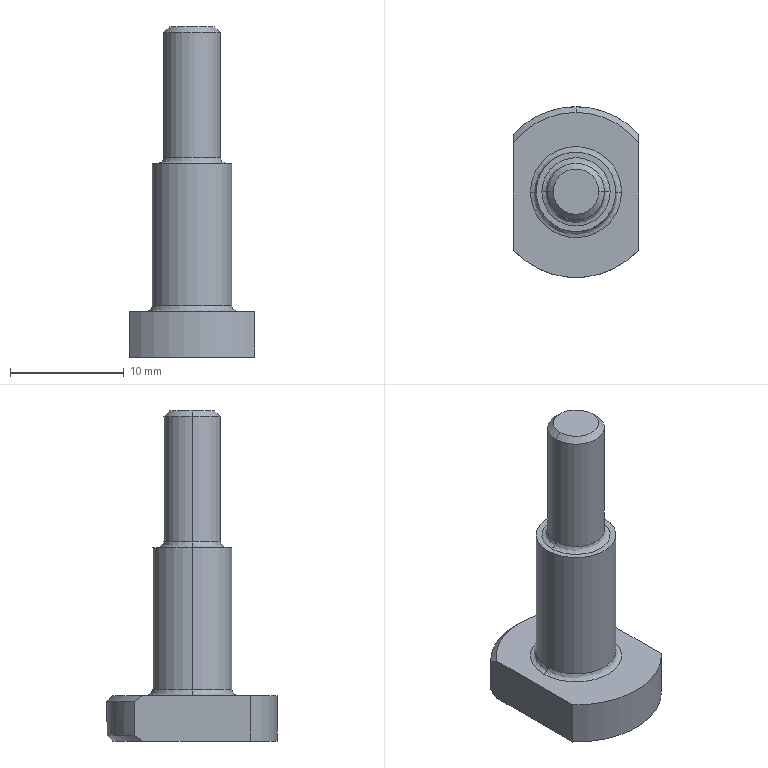Part | STEP file | Sensing post | 1 solid | 21 faces | box 11 x 15 x 29 mm | volume 1328 mm3 | cylinder 6 | plane 6 | cone 5 | spline 4 | commonest cylinder face diameters 5 x2 7 x2 15 x2